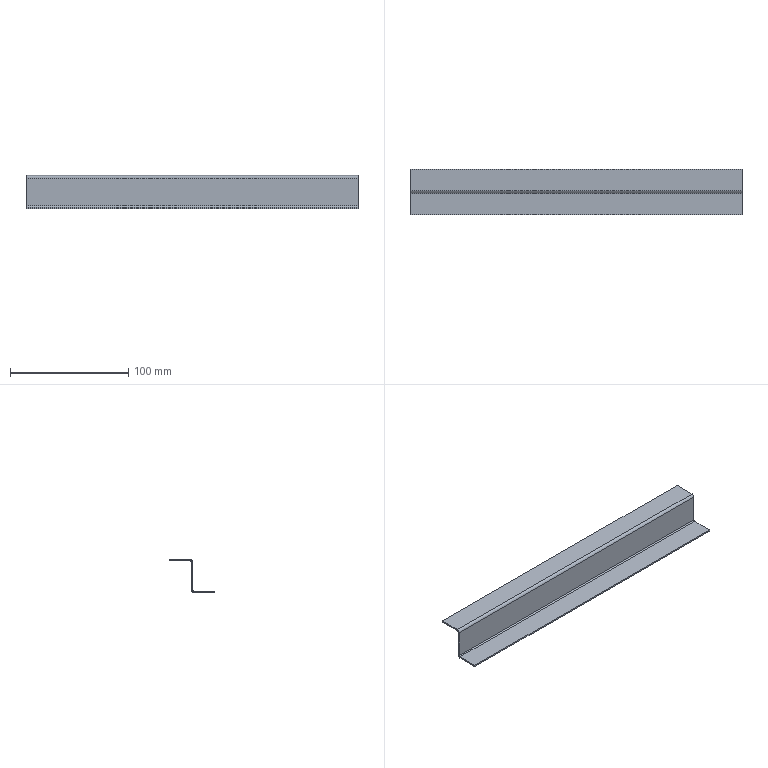Part | SolidWorks | features EdgeFlange 2, FlatPattern 1, HoleWzd 1, SMBaseFlange 1, SheetMetal 1 | 1 solid | 22 faces | box 281 x 38.8 x 28 mm | volume 21657 mm3 | plane 18 | cylinder 4 | commonest cylinder face diameters 2 x2 4.4 x2
STEP:
#1=CARTESIAN_POINT('',(140.5,10.,24.6));
#2=VERTEX_POINT('',#1);
#3=CARTESIAN_POINT('',(140.5,8.8,24.6));
#4=VERTEX_POINT('',#3);
#5=CARTESIAN_POINT('',(140.5,10.,24.6));
#6=DIRECTION('',(0.,-1.,0.));
#7=VECTOR('',#6,1000.);
#8=LINE('',#5,#7);
#9=EDGE_CURVE('',#2,#4,#8,.T.);
#10=ORIENTED_EDGE('',*,*,#9,.T.);
#11=CARTESIAN_POINT('',(140.5,8.8,1.));
#12=VERTEX_POINT('',#11);
#13=CARTESIAN_POINT('',(140.5,8.8,0.));
#14=DIRECTION('',(0.,0.,-1.));
#15=VECTOR('',#14,1000.);
#16=LINE('',#13,#15);
#17=EDGE_CURVE('',#4,#12,#16,.T.);
#18=ORIENTED_EDGE('',*,*,#17,.T.);
#19=CARTESIAN_POINT('',(140.5,10.,1.));
#20=VERTEX_POINT('',#19);
#21=CARTESIAN_POINT('',(140.5,10.,1.));
#22=DIRECTION('',(0.,1.,0.));
#23=VECTOR('',#22,1000.);
#24=LINE('',#21,#23);
#25=EDGE_CURVE('',#12,#20,#24,.T.);
#26=ORIENTED_EDGE('',*,*,#25,.T.);
#27=CARTESIAN_POINT('',(140.5,10.,0.));
#28=DIRECTION('',(0.,0.,-1.));
#29=VECTOR('',#28,1000.);
#30=LINE('',#27,#29);
#31=EDGE_CURVE('',#2,#20,#30,.T.);
#32=ORIENTED_EDGE('',*,*,#31,.F.);
#33=EDGE_LOOP('',(#10,#18,#26,#32));
#34=FACE_OUTER_BOUND('',#33,.T.);
#35=CARTESIAN_POINT('',(140.5,10.,0.));
#36=DIRECTION('',(-1.,0.,0.));
#37=DIRECTION('',(0.,0.,1.));
#38=AXIS2_PLACEMENT_3D('',#35,#36,#37);
#39=PLANE('',#38);
#40=ADVANCED_FACE('',(#34),#39,.F.);
#41=CARTESIAN_POINT('',(-140.5,10.,24.6));
#42=VERTEX_POINT('',#41);
#43=CARTESIAN_POINT('',(-140.5,8.8,24.6));
#44=VERTEX_POINT('',#43);
#45=CARTESIAN_POINT('',(-140.5,10.,24.6));
#46=DIRECTION('',(0.,-1.,0.));
#47=VECTOR('',#46,1000.);
#48=LINE('',#45,#47);
#49=EDGE_CURVE('',#42,#44,#48,.T.);
#50=ORIENTED_EDGE('',*,*,#49,.F.);
#51=CARTESIAN_POINT('',(-140.5,10.,1.));
#52=VERTEX_POINT('',#51);
#53=CARTESIAN_POINT('',(-140.5,10.,0.));
#54=DIRECTION('',(0.,0.,1.));
#55=VECTOR('',#54,1000.);
#56=LINE('',#53,#55);
#57=EDGE_CURVE('',#52,#42,#56,.T.);
#58=ORIENTED_EDGE('',*,*,#57,.F.);
#59=CARTESIAN_POINT('',(-140.5,8.8,1.));
#60=VERTEX_POINT('',#59);
#61=CARTESIAN_POINT('',(-140.5,8.8,1.));
#62=DIRECTION('',(0.,1.,0.));
#63=VECTOR('',#62,1000.);
#64=LINE('',#61,#63);
#65=EDGE_CURVE('',#60,#52,#64,.T.);
#66=ORIENTED_EDGE('',*,*,#65,.F.);
#67=CARTESIAN_POINT('',(-140.5,8.8,26.8));
#68=DIRECTION('',(0.,0.,1.));
#69=VECTOR('',#68,1000.);
#70=LINE('',#67,#69);
#71=EDGE_CURVE('',#60,#44,#70,.T.);
#72=ORIENTED_EDGE('',*,*,#71,.T.);
#73=EDGE_LOOP('',(#50,#58,#66,#72));
#74=FACE_OUTER_BOUND('',#73,.T.);
#75=CARTESIAN_POINT('',(-140.5,10.,26.8));
#76=DIRECTION('',(1.,0.,0.));
#77=DIRECTION('',(0.,0.,-1.));
#78=AXIS2_PLACEMENT_3D('',#75,#76,#77);
#79=PLANE('',#78);
#80=ADVANCED_FACE('',(#74),#79,.F.);
#81=CARTESIAN_POINT('',(140.5,10.,24.6));
#82=DIRECTION('',(-1.,0.,0.));
#83=VECTOR('',#82,1000.);
#84=LINE('',#81,#83);
#85=EDGE_CURVE('',#2,#42,#84,.T.);
#86=ORIENTED_EDGE('',*,*,#85,.F.);
#87=ORIENTED_EDGE('',*,*,#31,.T.);
#88=CARTESIAN_POINT('',(140.5,10.,1.));
#89=DIRECTION('',(1.,0.,0.));
#90=VECTOR('',#89,1000.);
#91=LINE('',#88,#90);
#92=EDGE_CURVE('',#52,#20,#91,.T.);
#93=ORIENTED_EDGE('',*,*,#92,.F.);
#94=ORIENTED_EDGE('',*,*,#57,.T.);
#95=EDGE_LOOP('',(#86,#87,#93,#94));
#96=FACE_OUTER_BOUND('',#95,.T.);
#97=CARTESIAN_POINT('',(0.,10.,0.));
#98=DIRECTION('',(0.,-1.,0.));
#99=DIRECTION('',(0.,0.,-1.));
#100=AXIS2_PLACEMENT_3D('',#97,#98,#99);
#101=PLANE('',#100);
#102=ADVANCED_FACE('',(#96),#101,.F.);
#103=ORIENTED_EDGE('',*,*,#17,.F.);
#104=CARTESIAN_POINT('',(140.5,8.8,24.6));
#105=DIRECTION('',(-1.,0.,0.));
#106=VECTOR('',#105,1000.);
#107=LINE('',#104,#106);
#108=EDGE_CURVE('',#4,#44,#107,.T.);
#109=ORIENTED_EDGE('',*,*,#108,.T.);
#110=ORIENTED_EDGE('',*,*,#71,.F.);
#111=CARTESIAN_POINT('',(140.5,8.8,1.));
#112=DIRECTION('',(-1.,0.,0.));
#113=VECTOR('',#112,1000.);
#114=LINE('',#111,#113);
#115=EDGE_CURVE('',#12,#60,#114,.T.);
#116=ORIENTED_EDGE('',*,*,#115,.F.);
#117=EDGE_LOOP('',(#103,#109,#110,#116));
#118=FACE_OUTER_BOUND('',#117,.T.);
#119=CARTESIAN_POINT('',(0.,8.8,0.));
#120=DIRECTION('',(0.,-1.,0.));
#121=DIRECTION('',(0.,0.,-1.));
#122=AXIS2_PLACEMENT_3D('',#119,#120,#121);
#123=PLANE('',#122);
#124=ADVANCED_FACE('',(#118),#123,.T.);
#125=CARTESIAN_POINT('',(-140.5,7.8,0.));
#126=VERTEX_POINT('',#125);
#127=CARTESIAN_POINT('',(-140.5,-10.,0.));
#128=VERTEX_POINT('',#127);
#129=CARTESIAN_POINT('',(-140.5,10.,0.));
#130=DIRECTION('',(0.,-1.,0.));
#131=VECTOR('',#130,1000.);
#132=LINE('',#129,#131);
#133=EDGE_CURVE('',#126,#128,#132,.T.);
#134=ORIENTED_EDGE('',*,*,#133,.F.);
#135=CARTESIAN_POINT('',(-140.5,7.8,-1.2));
#136=VERTEX_POINT('',#135);
#137=CARTESIAN_POINT('',(-140.5,7.8,0.));
#138=DIRECTION('',(0.,0.,-1.));
#139=VECTOR('',#138,1000.);
#140=LINE('',#137,#139);
#141=EDGE_CURVE('',#126,#136,#140,.T.);
#142=ORIENTED_EDGE('',*,*,#141,.T.);
#143=CARTESIAN_POINT('',(-140.5,-10.,-1.2));
#144=VERTEX_POINT('',#143);
#145=CARTESIAN_POINT('',(-140.5,10.,-1.2));
#146=DIRECTION('',(0.,-1.,0.));
#147=VECTOR('',#146,1000.);
#148=LINE('',#145,#147);
#149=EDGE_CURVE('',#136,#144,#148,.T.);
#150=ORIENTED_EDGE('',*,*,#149,.T.);
#151=CARTESIAN_POINT('',(-140.5,-10.,-1.2));
#152=DIRECTION('',(0.,0.,1.));
#153=VECTOR('',#152,1000.);
#154=LINE('',#151,#153);
#155=EDGE_CURVE('',#144,#128,#154,.T.);
#156=ORIENTED_EDGE('',*,*,#155,.T.);
#157=EDGE_LOOP('',(#134,#142,#150,#156));
#158=FACE_OUTER_BOUND('',#157,.T.);
#159=CARTESIAN_POINT('',(-140.5,10.,-1.2));
#160=DIRECTION('',(-1.,0.,0.));
#161=DIRECTION('',(0.,0.,1.));
#162=AXIS2_PLACEMENT_3D('',#159,#160,#161);
#163=PLANE('',#162);
#164=ADVANCED_FACE('',(#158),#163,.T.);
#165=CARTESIAN_POINT('',(140.5,7.8,-1.2));
#166=VERTEX_POINT('',#165);
#167=CARTESIAN_POINT('',(-140.5,7.8,-1.2));
#168=DIRECTION('',(1.,0.,0.));
#169=VECTOR('',#168,1000.);
#170=LINE('',#167,#169);
#171=EDGE_CURVE('',#136,#166,#170,.T.);
#172=ORIENTED_EDGE('',*,*,#171,.T.);
#173=CARTESIAN_POINT('',(140.5,-10.,-1.2));
#174=VERTEX_POINT('',#173);
#175=CARTESIAN_POINT('',(140.5,10.,-1.2));
#176=DIRECTION('',(0.,1.,0.));
#177=VECTOR('',#176,1000.);
#178=LINE('',#175,#177);
#179=EDGE_CURVE('',#174,#166,#178,.T.);
#180=ORIENTED_EDGE('',*,*,#179,.F.);
#181=CARTESIAN_POINT('',(-140.5,-10.,-1.2));
#182=DIRECTION('',(1.,0.,0.));
#183=VECTOR('',#182,1000.);
#184=LINE('',#181,#183);
#185=EDGE_CURVE('',#144,#174,#184,.T.);
#186=ORIENTED_EDGE('',*,*,#185,.F.);
#187=ORIENTED_EDGE('',*,*,#149,.F.);
#188=EDGE_LOOP('',(#172,#180,#186,#187));
#189=FACE_OUTER_BOUND('',#188,.T.);
#190=CARTESIAN_POINT('',(0.,0.,-1.2));
#191=DIRECTION('',(0.,0.,1.));
#192=DIRECTION('',(1.,0.,0.));
#193=AXIS2_PLACEMENT_3D('',#190,#191,#192);
#194=PLANE('',#193);
#195=ADVANCED_FACE('',(#189),#194,.F.);
#196=CARTESIAN_POINT('',(140.5,-10.,0.));
#197=VERTEX_POINT('',#196);
#198=CARTESIAN_POINT('',(140.5,7.8,0.));
#199=VERTEX_POINT('',#198);
#200=CARTESIAN_POINT('',(140.5,10.,0.));
#201=DIRECTION('',(0.,1.,0.));
#202=VECTOR('',#201,1000.);
#203=LINE('',#200,#202);
#204=EDGE_CURVE('',#197,#199,#203,.T.);
#205=ORIENTED_EDGE('',*,*,#204,.T.);
#206=CARTESIAN_POINT('',(-140.5,7.8,0.));
#207=DIRECTION('',(1.,0.,0.));
#208=VECTOR('',#207,1000.);
#209=LINE('',#206,#208);
#210=EDGE_CURVE('',#126,#199,#209,.T.);
#211=ORIENTED_EDGE('',*,*,#210,.F.);
#212=ORIENTED_EDGE('',*,*,#133,.T.);
#213=CARTESIAN_POINT('',(-140.5,-10.,0.));
#214=DIRECTION('',(1.,0.,0.));
#215=VECTOR('',#214,1000.);
#216=LINE('',#213,#215);
#217=EDGE_CURVE('',#128,#197,#216,.T.);
#218=ORIENTED_EDGE('',*,*,#217,.T.);
#219=EDGE_LOOP('',(#205,#211,#212,#218));
#220=FACE_OUTER_BOUND('',#219,.T.);
#221=CARTESIAN_POINT('',(0.,0.,0.));
#222=DIRECTION('',(0.,0.,1.));
#223=DIRECTION('',(1.,0.,0.));
#224=AXIS2_PLACEMENT_3D('',#221,#222,#223);
#225=PLANE('',#224);
#226=ADVANCED_FACE('',(#220),#225,.T.);
#227=CARTESIAN_POINT('',(140.5,7.8,0.));
#228=DIRECTION('',(0.,0.,-1.));
#229=VECTOR('',#228,1000.);
#230=LINE('',#227,#229);
#231=EDGE_CURVE('',#199,#166,#230,.T.);
#232=ORIENTED_EDGE('',*,*,#231,.F.);
#233=ORIENTED_EDGE('',*,*,#204,.F.);
#234=CARTESIAN_POINT('',(140.5,-10.,-1.2));
#235=DIRECTION('',(0.,0.,1.));
#236=VECTOR('',#235,1000.);
#237=LINE('',#234,#236);
#238=EDGE_CURVE('',#174,#197,#237,.T.);
#239=ORIENTED_EDGE('',*,*,#238,.F.);
#240=ORIENTED_EDGE('',*,*,#179,.T.);
#241=EDGE_LOOP('',(#232,#233,#239,#240));
#242=FACE_OUTER_BOUND('',#241,.T.);
#243=CARTESIAN_POINT('',(140.5,10.,-1.2));
#244=DIRECTION('',(1.,0.,0.));
#245=DIRECTION('',(0.,0.,-1.));
#246=AXIS2_PLACEMENT_3D('',#243,#244,#245);
#247=PLANE('',#246);
#248=ADVANCED_FACE('',(#242),#247,.T.);
#249=ORIENTED_EDGE('',*,*,#217,.F.);
#250=ORIENTED_EDGE('',*,*,#155,.F.);
#251=ORIENTED_EDGE('',*,*,#185,.T.);
#252=ORIENTED_EDGE('',*,*,#238,.T.);
#253=EDGE_LOOP('',(#249,#250,#251,#252));
#254=FACE_OUTER_BOUND('',#253,.T.);
#255=CARTESIAN_POINT('',(-140.5,-10.,-1.2));
#256=DIRECTION('',(0.,-1.,0.));
#257=DIRECTION('',(0.,0.,-1.));
#258=AXIS2_PLACEMENT_3D('',#255,#256,#257);
#259=PLANE('',#258);
#260=ADVANCED_FACE('',(#254),#259,.T.);
#261=ORIENTED_EDGE('',*,*,#25,.F.);
#262=CARTESIAN_POINT('',(140.5,7.8,1.));
#263=DIRECTION('',(1.,0.,0.));
#264=DIRECTION('',(0.,0.,1.));
#265=AXIS2_PLACEMENT_3D('',#262,#263,#264);
#266=CIRCLE('',#265,1.);
#267=EDGE_CURVE('',#199,#12,#266,.T.);
#268=ORIENTED_EDGE('',*,*,#267,.F.);
#269=ORIENTED_EDGE('',*,*,#231,.T.);
#270=CARTESIAN_POINT('',(140.5,7.8,1.));
#271=DIRECTION('',(1.,0.,0.));
#272=DIRECTION('',(0.,0.,1.));
#273=AXIS2_PLACEMENT_3D('',#270,#271,#272);
#274=CIRCLE('',#273,2.2);
#275=EDGE_CURVE('',#166,#20,#274,.T.);
#276=ORIENTED_EDGE('',*,*,#275,.T.);
#277=EDGE_LOOP('',(#261,#268,#269,#276));
#278=FACE_OUTER_BOUND('',#277,.T.);
#279=CARTESIAN_POINT('',(140.5,7.8,1.));
#280=DIRECTION('',(1.,0.,0.));
#281=DIRECTION('',(0.,0.,-1.));
#282=AXIS2_PLACEMENT_3D('',#279,#280,#281);
#283=PLANE('',#282);
#284=ADVANCED_FACE('',(#278),#283,.T.);
#285=CARTESIAN_POINT('',(-140.5,7.8,1.));
#286=DIRECTION('',(-1.,0.,0.));
#287=DIRECTION('',(0.,0.,1.));
#288=AXIS2_PLACEMENT_3D('',#285,#286,#287);
#289=CIRCLE('',#288,1.);
#290=EDGE_CURVE('',#60,#126,#289,.T.);
#291=ORIENTED_EDGE('',*,*,#290,.F.);
#292=ORIENTED_EDGE('',*,*,#65,.T.);
#293=CARTESIAN_POINT('',(-140.5,7.8,1.));
#294=DIRECTION('',(-1.,0.,0.));
#295=DIRECTION('',(0.,0.,1.));
#296=AXIS2_PLACEMENT_3D('',#293,#294,#295);
#297=CIRCLE('',#296,2.2);
#298=EDGE_CURVE('',#52,#136,#297,.T.);
#299=ORIENTED_EDGE('',*,*,#298,.T.);
#300=ORIENTED_EDGE('',*,*,#141,.F.);
#301=EDGE_LOOP('',(#291,#292,#299,#300));
#302=FACE_OUTER_BOUND('',#301,.T.);
#303=CARTESIAN_POINT('',(-140.5,7.8,1.));
#304=DIRECTION('',(1.,0.,0.));
#305=DIRECTION('',(0.,0.,-1.));
#306=AXIS2_PLACEMENT_3D('',#303,#304,#305);
#307=PLANE('',#306);
#308=ADVANCED_FACE('',(#302),#307,.F.);
#309=ORIENTED_EDGE('',*,*,#171,.F.);
#310=ORIENTED_EDGE('',*,*,#298,.F.);
#311=ORIENTED_EDGE('',*,*,#92,.T.);
#312=ORIENTED_EDGE('',*,*,#275,.F.);
#313=EDGE_LOOP('',(#309,#310,#311,#312));
#314=FACE_OUTER_BOUND('',#313,.T.);
#315=CARTESIAN_POINT('',(-140.5,7.8,1.));
#316=DIRECTION('',(-1.,0.,0.));
#317=DIRECTION('',(0.,1.,0.));
#318=AXIS2_PLACEMENT_3D('',#315,#316,#317);
#319=CYLINDRICAL_SURFACE('',#318,2.2);
#320=ADVANCED_FACE('',(#314),#319,.T.);
#321=ORIENTED_EDGE('',*,*,#210,.T.);
#322=ORIENTED_EDGE('',*,*,#267,.T.);
#323=ORIENTED_EDGE('',*,*,#115,.T.);
#324=ORIENTED_EDGE('',*,*,#290,.T.);
#325=EDGE_LOOP('',(#321,#322,#323,#324));
#326=FACE_OUTER_BOUND('',#325,.T.);
#327=CARTESIAN_POINT('',(-140.5,7.8,1.));
#328=DIRECTION('',(-1.,0.,0.));
#329=DIRECTION('',(0.,1.,0.));
#330=AXIS2_PLACEMENT_3D('',#327,#328,#329);
#331=CYLINDRICAL_SURFACE('',#330,1.);
#332=ADVANCED_FACE('',(#326),#331,.F.);
#333=CARTESIAN_POINT('',(-140.5,11.,25.6));
#334=VERTEX_POINT('',#333);
#335=CARTESIAN_POINT('',(-140.5,11.,26.8));
#336=VERTEX_POINT('',#335);
#337=CARTESIAN_POINT('',(-140.5,11.,26.8));
#338=DIRECTION('',(0.,0.,1.));
#339=VECTOR('',#338,1000.);
#340=LINE('',#337,#339);
#341=EDGE_CURVE('',#334,#336,#340,.T.);
#342=ORIENTED_EDGE('',*,*,#341,.F.);
#343=CARTESIAN_POINT('',(-140.5,11.,24.6));
#344=DIRECTION('',(-1.,0.,0.));
#345=DIRECTION('',(0.,0.,-1.));
#346=AXIS2_PLACEMENT_3D('',#343,#344,#345);
#347=CIRCLE('',#346,1.);
#348=EDGE_CURVE('',#42,#334,#347,.T.);
#349=ORIENTED_EDGE('',*,*,#348,.F.);
#350=ORIENTED_EDGE('',*,*,#49,.T.);
#351=CARTESIAN_POINT('',(-140.5,11.,24.6));
#352=DIRECTION('',(-1.,0.,0.));
#353=DIRECTION('',(0.,0.,-1.));
#354=AXIS2_PLACEMENT_3D('',#351,#352,#353);
#355=CIRCLE('',#354,2.2);
#356=EDGE_CURVE('',#44,#336,#355,.T.);
#357=ORIENTED_EDGE('',*,*,#356,.T.);
#358=EDGE_LOOP('',(#342,#349,#350,#357));
#359=FACE_OUTER_BOUND('',#358,.T.);
#360=CARTESIAN_POINT('',(-140.5,11.,24.6));
#361=DIRECTION('',(-1.,0.,0.));
#362=DIRECTION('',(0.,0.,1.));
#363=AXIS2_PLACEMENT_3D('',#360,#361,#362);
#364=PLANE('',#363);
#365=ADVANCED_FACE('',(#359),#364,.T.);
#366=CARTESIAN_POINT('',(140.5,11.,25.6));
#367=VERTEX_POINT('',#366);
#368=CARTESIAN_POINT('',(140.5,11.,24.6));
#369=DIRECTION('',(1.,0.,0.));
#370=DIRECTION('',(0.,0.,-1.));
#371=AXIS2_PLACEMENT_3D('',#368,#369,#370);
#372=CIRCLE('',#371,1.);
#373=EDGE_CURVE('',#367,#2,#372,.T.);
#374=ORIENTED_EDGE('',*,*,#373,.F.);
#375=CARTESIAN_POINT('',(140.5,11.,26.8));
#376=VERTEX_POINT('',#375);
#377=CARTESIAN_POINT('',(140.5,11.,25.6));
#378=DIRECTION('',(0.,0.,1.));
#379=VECTOR('',#378,1000.);
#380=LINE('',#377,#379);
#381=EDGE_CURVE('',#367,#376,#380,.T.);
#382=ORIENTED_EDGE('',*,*,#381,.T.);
#383=CARTESIAN_POINT('',(140.5,11.,24.6));
#384=DIRECTION('',(1.,0.,0.));
#385=DIRECTION('',(0.,0.,-1.));
#386=AXIS2_PLACEMENT_3D('',#383,#384,#385);
#387=CIRCLE('',#386,2.2);
#388=EDGE_CURVE('',#376,#4,#387,.T.);
#389=ORIENTED_EDGE('',*,*,#388,.T.);
#390=ORIENTED_EDGE('',*,*,#9,.F.);
#391=EDGE_LOOP('',(#374,#382,#389,#390));
#392=FACE_OUTER_BOUND('',#391,.T.);
#393=CARTESIAN_POINT('',(140.5,11.,24.6));
#394=DIRECTION('',(-1.,0.,0.));
#395=DIRECTION('',(0.,0.,1.));
#396=AXIS2_PLACEMENT_3D('',#393,#394,#395);
#397=PLANE('',#396);
#398=ADVANCED_FACE('',(#392),#397,.F.);
#399=ORIENTED_EDGE('',*,*,#108,.F.);
#400=ORIENTED_EDGE('',*,*,#388,.F.);
#401=CARTESIAN_POINT('',(-140.5,11.,26.8));
#402=DIRECTION('',(-1.,0.,0.));
#403=VECTOR('',#402,1000.);
#404=LINE('',#401,#403);
#405=EDGE_CURVE('',#376,#336,#404,.T.);
#406=ORIENTED_EDGE('',*,*,#405,.T.);
#407=ORIENTED_EDGE('',*,*,#356,.F.);
#408=EDGE_LOOP('',(#399,#400,#406,#407));
#409=FACE_OUTER_BOUND('',#408,.T.);
#410=CARTESIAN_POINT('',(140.5,11.,24.6));
#411=DIRECTION('',(1.,0.,0.));
#412=DIRECTION('',(0.,0.,1.));
#413=AXIS2_PLACEMENT_3D('',#410,#411,#412);
#414=CYLINDRICAL_SURFACE('',#413,2.2);
#415=ADVANCED_FACE('',(#409),#414,.T.);
#416=ORIENTED_EDGE('',*,*,#85,.T.);
#417=ORIENTED_EDGE('',*,*,#348,.T.);
#418=CARTESIAN_POINT('',(-140.5,11.,25.6));
#419=DIRECTION('',(1.,0.,0.));
#420=VECTOR('',#419,1000.);
#421=LINE('',#418,#420);
#422=EDGE_CURVE('',#334,#367,#421,.T.);
#423=ORIENTED_EDGE('',*,*,#422,.T.);
#424=ORIENTED_EDGE('',*,*,#373,.T.);
#425=EDGE_LOOP('',(#416,#417,#423,#424));
#426=FACE_OUTER_BOUND('',#425,.T.);
#427=CARTESIAN_POINT('',(140.5,11.,24.6));
#428=DIRECTION('',(1.,0.,0.));
#429=DIRECTION('',(0.,0.,1.));
#430=AXIS2_PLACEMENT_3D('',#427,#428,#429);
#431=CYLINDRICAL_SURFACE('',#430,1.);
#432=ADVANCED_FACE('',(#426),#431,.F.);
#433=ORIENTED_EDGE('',*,*,#341,.T.);
#434=CARTESIAN_POINT('',(-140.5,28.8,26.8));
#435=VERTEX_POINT('',#434);
#436=CARTESIAN_POINT('',(-140.5,0.,26.8));
#437=DIRECTION('',(0.,-1.,0.));
#438=VECTOR('',#437,1000.);
#439=LINE('',#436,#438);
#440=EDGE_CURVE('',#435,#336,#439,.T.);
#441=ORIENTED_EDGE('',*,*,#440,.F.);
#442=CARTESIAN_POINT('',(-140.5,28.8,25.6));
#443=VERTEX_POINT('',#442);
#444=CARTESIAN_POINT('',(-140.5,28.8,26.8));
#445=DIRECTION('',(0.,0.,-1.));
#446=VECTOR('',#445,1000.);
#447=LINE('',#444,#446);
#448=EDGE_CURVE('',#435,#443,#447,.T.);
#449=ORIENTED_EDGE('',*,*,#448,.T.);
#450=CARTESIAN_POINT('',(-140.5,10.,25.6));
#451=DIRECTION('',(0.,-1.,0.));
#452=VECTOR('',#451,1000.);
#453=LINE('',#450,#452);
#454=EDGE_CURVE('',#443,#334,#453,.T.);
#455=ORIENTED_EDGE('',*,*,#454,.T.);
#456=EDGE_LOOP('',(#433,#441,#449,#455));
#457=FACE_OUTER_BOUND('',#456,.T.);
#458=CARTESIAN_POINT('',(-140.5,10.,26.8));
#459=DIRECTION('',(1.,0.,0.));
#460=DIRECTION('',(0.,0.,-1.));
#461=AXIS2_PLACEMENT_3D('',#458,#459,#460);
#462=PLANE('',#461);
#463=ADVANCED_FACE('',(#457),#462,.F.);
#464=ORIENTED_EDGE('',*,*,#381,.F.);
#465=CARTESIAN_POINT('',(140.5,28.8,25.6));
#466=VERTEX_POINT('',#465);
#467=CARTESIAN_POINT('',(140.5,28.8,25.6));
#468=DIRECTION('',(0.,1.,0.));
#469=VECTOR('',#468,1000.);
#470=LINE('',#467,#469);
#471=EDGE_CURVE('',#367,#466,#470,.T.);
#472=ORIENTED_EDGE('',*,*,#471,.T.);
#473=CARTESIAN_POINT('',(140.5,28.8,26.8));
#474=VERTEX_POINT('',#473);
#475=CARTESIAN_POINT('',(140.5,28.8,26.8));
#476=DIRECTION('',(0.,0.,-1.));
#477=VECTOR('',#476,1000.);
#478=LINE('',#475,#477);
#479=EDGE_CURVE('',#474,#466,#478,.T.);
#480=ORIENTED_EDGE('',*,*,#479,.F.);
#481=CARTESIAN_POINT('',(140.5,0.,26.8));
#482=DIRECTION('',(0.,1.,0.));
#483=VECTOR('',#482,1000.);
#484=LINE('',#481,#483);
#485=EDGE_CURVE('',#376,#474,#484,.T.);
#486=ORIENTED_EDGE('',*,*,#485,.F.);
#487=EDGE_LOOP('',(#464,#472,#480,#486));
#488=FACE_OUTER_BOUND('',#487,.T.);
#489=CARTESIAN_POINT('',(140.5,28.8,26.8));
#490=DIRECTION('',(-1.,0.,0.));
#491=DIRECTION('',(0.,0.,1.));
#492=AXIS2_PLACEMENT_3D('',#489,#490,#491);
#493=PLANE('',#492);
#494=ADVANCED_FACE('',(#488),#493,.F.);
#495=ORIENTED_EDGE('',*,*,#405,.F.);
#496=ORIENTED_EDGE('',*,*,#485,.T.);
#497=CARTESIAN_POINT('',(0.,28.8,26.8));
#498=DIRECTION('',(-1.,0.,0.));
#499=VECTOR('',#498,1000.);
#500=LINE('',#497,#499);
#501=EDGE_CURVE('',#474,#435,#500,.T.);
#502=ORIENTED_EDGE('',*,*,#501,.T.);
#503=ORIENTED_EDGE('',*,*,#440,.T.);
#504=EDGE_LOOP('',(#495,#496,#502,#503));
#505=FACE_OUTER_BOUND('',#504,.T.);
#506=CARTESIAN_POINT('',(0.,0.,26.8));
#507=DIRECTION('',(0.,0.,-1.));
#508=DIRECTION('',(-1.,0.,0.));
#509=AXIS2_PLACEMENT_3D('',#506,#507,#508);
#510=PLANE('',#509);
#511=ADVANCED_FACE('',(#505),#510,.F.);
#512=ORIENTED_EDGE('',*,*,#471,.F.);
#513=ORIENTED_EDGE('',*,*,#422,.F.);
#514=ORIENTED_EDGE('',*,*,#454,.F.);
#515=CARTESIAN_POINT('',(-140.5,28.8,25.6));
#516=DIRECTION('',(-1.,0.,0.));
#517=VECTOR('',#516,1000.);
#518=LINE('',#515,#517);
#519=EDGE_CURVE('',#466,#443,#518,.T.);
#520=ORIENTED_EDGE('',*,*,#519,.F.);
#521=EDGE_LOOP('',(#512,#513,#514,#520));
#522=FACE_OUTER_BOUND('',#521,.T.);
#523=CARTESIAN_POINT('',(0.,0.,25.6));
#524=DIRECTION('',(0.,0.,-1.));
#525=DIRECTION('',(-1.,0.,0.));
#526=AXIS2_PLACEMENT_3D('',#523,#524,#525);
#527=PLANE('',#526);
#528=ADVANCED_FACE('',(#522),#527,.T.);
#529=ORIENTED_EDGE('',*,*,#519,.T.);
#530=ORIENTED_EDGE('',*,*,#448,.F.);
#531=ORIENTED_EDGE('',*,*,#501,.F.);
#532=ORIENTED_EDGE('',*,*,#479,.T.);
#533=EDGE_LOOP('',(#529,#530,#531,#532));
#534=FACE_OUTER_BOUND('',#533,.T.);
#535=CARTESIAN_POINT('',(-140.5,28.8,26.8));
#536=DIRECTION('',(0.,-1.,0.));
#537=DIRECTION('',(0.,0.,-1.));
#538=AXIS2_PLACEMENT_3D('',#535,#536,#537);
#539=PLANE('',#538);
#540=ADVANCED_FACE('',(#534),#539,.F.);
#541=CLOSED_SHELL('',(#40,#80,#102,#124,#164,#195,#226,#248,#260,#284,#308,#320,#332,#365,#398,#415,#432,#463,#494,#511,#528,#540));
#542=MANIFOLD_SOLID_BREP('',#541);
#543=CARTESIAN_POINT('',(0.,0.,0.));
#544=DIRECTION('',(0.,0.,1.));
#545=DIRECTION('',(1.,0.,0.));
#546=AXIS2_PLACEMENT_3D('',#543,#544,#545);
#547=(LENGTH_UNIT()NAMED_UNIT(*)SI_UNIT(.MILLI.,.METRE.));
#548=UNCERTAINTY_MEASURE_WITH_UNIT(LENGTH_MEASURE(0.00001),#547,'','');
#549=(NAMED_UNIT(*)PLANE_ANGLE_UNIT()SI_UNIT($,.RADIAN.));
#550=(NAMED_UNIT(*)SI_UNIT($,.STERADIAN.)SOLID_ANGLE_UNIT());
#551=(GEOMETRIC_REPRESENTATION_CONTEXT(3)GLOBAL_UNCERTAINTY_ASSIGNED_CONTEXT((#548))GLOBAL_UNIT_ASSIGNED_CONTEXT((#547,#549,#550))REPRESENTATION_CONTEXT('',''));
#552=ADVANCED_BREP_SHAPE_REPRESENTATION('',(#542,#546),#551);